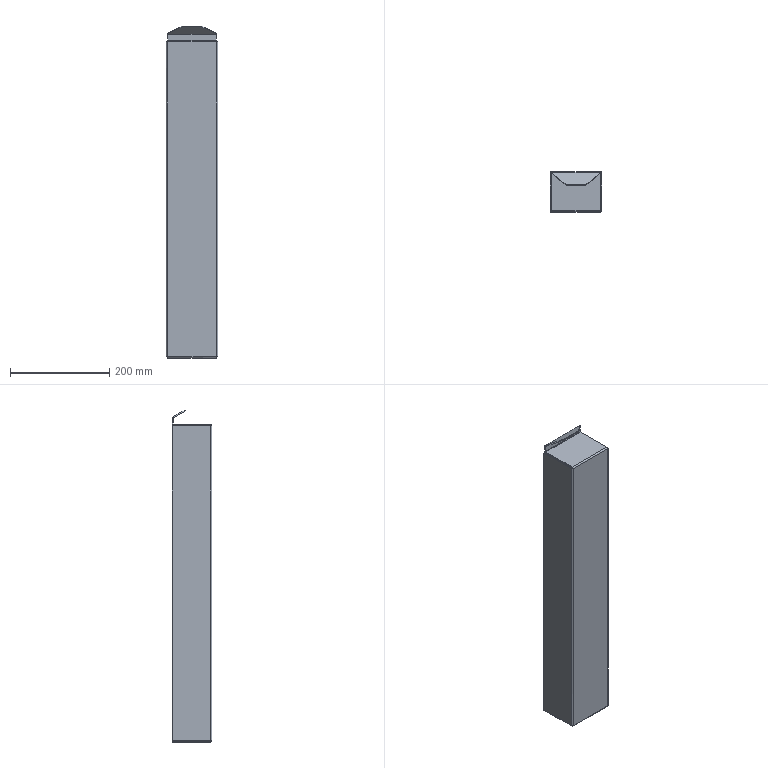Part | SolidWorks | features EdgeFlange 3, FlatPattern 1, ICE 1, SMBaseFlange 1, SheetMetal 1 | 1 solid | 54 faces | box 104 x 80 x 668.155 mm | volume 365737 mm3 | plane 34 | cylinder 12 | spline 8 | commonest cylinder face diameters 1.473 x6 5.473 x6